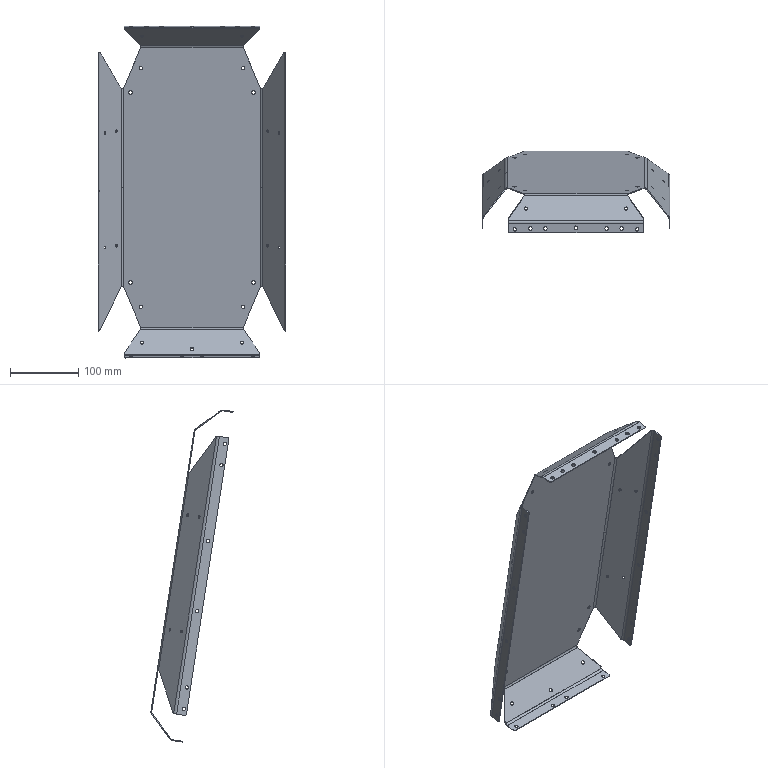Part | SolidWorks | features BaseBody 1 | 1 solid | 184 faces | box 275 x 120.427 x 486.513 mm | volume 183360 mm3 | cylinder 126 | plane 54 | spline 4 | commonest cylinder face diameters 4.9 x38 5.2 x34 4 x24 10 x12 12.4 x10 8 x8